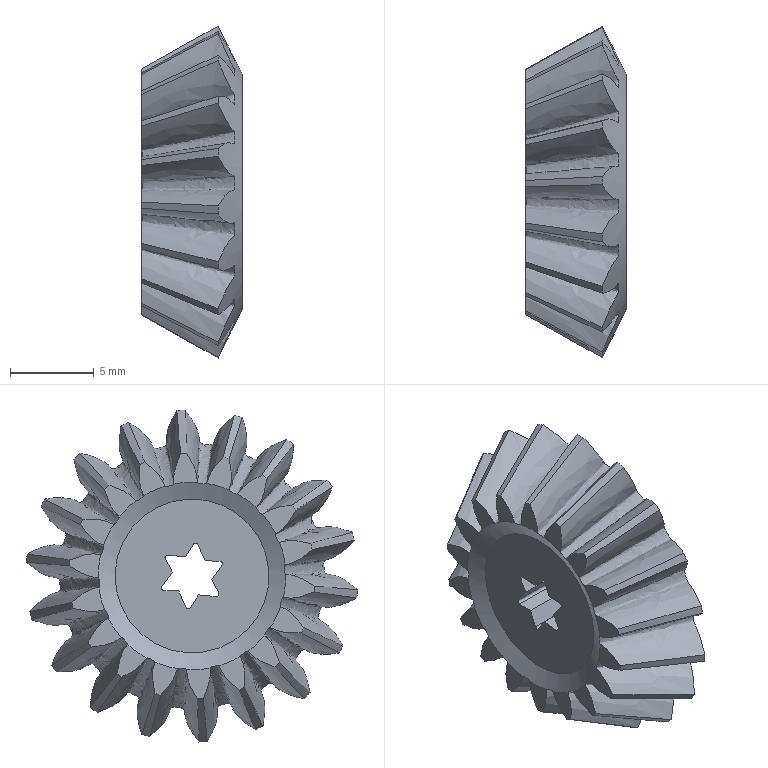Part | STEP file | Wytnij-wyci_gni_cie1_3 | 1 solid | 78 faces | box 6 x 19.721 x 19.771 mm | volume 1055 mm3 | plane 32 | spline 30 | cone 8 | cylinder 8 | commonest cylinder face diameters 0.3 x8